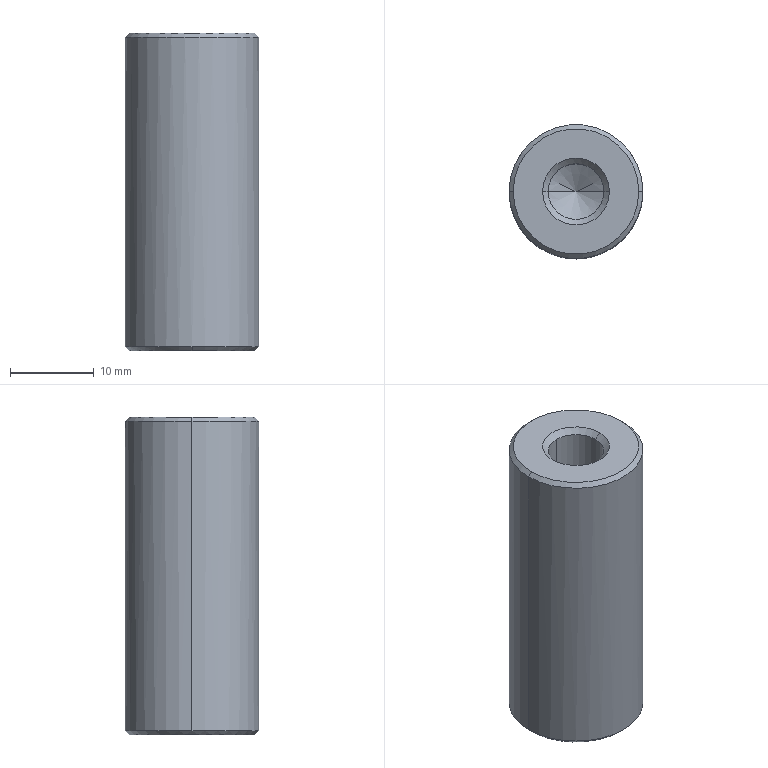Part | SolidWorks | features BaseBody 1 | 1 solid | 14 faces | box 16 x 16 x 38 mm | volume 7208 mm3 | cone 8 | cylinder 4 | plane 2 | commonest cylinder face diameters 6.647 x2 16 x2
STEP:
#1=CARTESIAN_POINT('',(0.,8.,-18.5));
#2=VERTEX_POINT('',#1);
#3=CARTESIAN_POINT('',(-8.,0.,-18.5));
#4=VERTEX_POINT('',#3);
#5=CARTESIAN_POINT('',(0.,0.,-18.5));
#6=DIRECTION('',(0.,0.,1.));
#7=DIRECTION('',(1.,0.,0.));
#8=AXIS2_PLACEMENT_3D('',#5,#6,#7);
#9=CIRCLE('',#8,8.);
#10=EDGE_CURVE('',#2,#4,#9,.T.);
#11=ORIENTED_EDGE('',*,*,#10,.T.);
#12=CARTESIAN_POINT('',(-8.,0.,18.5));
#13=VERTEX_POINT('',#12);
#14=CARTESIAN_POINT('',(-8.,0.,-19.));
#15=DIRECTION('',(0.,0.,1.));
#16=VECTOR('',#15,1000.);
#17=LINE('',#14,#16);
#18=EDGE_CURVE('',#4,#13,#17,.T.);
#19=ORIENTED_EDGE('',*,*,#18,.T.);
#20=CARTESIAN_POINT('',(8.,0.,18.5));
#21=VERTEX_POINT('',#20);
#22=CARTESIAN_POINT('',(0.,0.,18.5));
#23=DIRECTION('',(0.,0.,-1.));
#24=DIRECTION('',(1.,0.,0.));
#25=AXIS2_PLACEMENT_3D('',#22,#23,#24);
#26=CIRCLE('',#25,8.);
#27=EDGE_CURVE('',#13,#21,#26,.T.);
#28=ORIENTED_EDGE('',*,*,#27,.T.);
#29=CARTESIAN_POINT('',(8.,0.,-18.5));
#30=VERTEX_POINT('',#29);
#31=CARTESIAN_POINT('',(8.,0.,-19.));
#32=DIRECTION('',(0.,0.,1.));
#33=VECTOR('',#32,1000.);
#34=LINE('',#31,#33);
#35=EDGE_CURVE('',#30,#21,#34,.T.);
#36=ORIENTED_EDGE('',*,*,#35,.F.);
#37=CARTESIAN_POINT('',(0.,0.,-18.5));
#38=DIRECTION('',(0.,0.,1.));
#39=DIRECTION('',(1.,0.,0.));
#40=AXIS2_PLACEMENT_3D('',#37,#38,#39);
#41=CIRCLE('',#40,8.);
#42=EDGE_CURVE('',#30,#2,#41,.T.);
#43=ORIENTED_EDGE('',*,*,#42,.T.);
#44=EDGE_LOOP('',(#11,#19,#28,#36,#43));
#45=FACE_OUTER_BOUND('',#44,.T.);
#46=CARTESIAN_POINT('',(0.,0.,-19.));
#47=DIRECTION('',(0.,0.,1.));
#48=DIRECTION('',(1.,0.,0.));
#49=AXIS2_PLACEMENT_3D('',#46,#47,#48);
#50=CYLINDRICAL_SURFACE('',#49,8.);
#51=ADVANCED_FACE('',(#45),#50,.T.);
#52=CARTESIAN_POINT('',(-7.5,0.,19.));
#53=VERTEX_POINT('',#52);
#54=CARTESIAN_POINT('',(7.5,0.,19.));
#55=VERTEX_POINT('',#54);
#56=CARTESIAN_POINT('',(0.,0.,19.));
#57=DIRECTION('',(0.,0.,-1.));
#58=DIRECTION('',(-1.,0.,0.));
#59=AXIS2_PLACEMENT_3D('',#56,#57,#58);
#60=CIRCLE('',#59,7.5);
#61=EDGE_CURVE('',#53,#55,#60,.T.);
#62=ORIENTED_EDGE('',*,*,#61,.T.);
#63=CARTESIAN_POINT('',(8.,0.,18.5));
#64=DIRECTION('',(0.7071,0.,-0.7071));
#65=VECTOR('',#64,1000.);
#66=LINE('',#63,#65);
#67=EDGE_CURVE('',#55,#21,#66,.T.);
#68=ORIENTED_EDGE('',*,*,#67,.T.);
#69=ORIENTED_EDGE('',*,*,#27,.F.);
#70=CARTESIAN_POINT('',(-8.,0.,18.5));
#71=DIRECTION('',(-0.7071,0.,-0.7071));
#72=VECTOR('',#71,1000.);
#73=LINE('',#70,#72);
#74=EDGE_CURVE('',#53,#13,#73,.T.);
#75=ORIENTED_EDGE('',*,*,#74,.F.);
#76=EDGE_LOOP('',(#62,#68,#69,#75));
#77=FACE_OUTER_BOUND('',#76,.T.);
#78=CARTESIAN_POINT('',(0.,0.,18.5));
#79=DIRECTION('',(0.,0.,-1.));
#80=DIRECTION('',(-1.,0.,0.));
#81=AXIS2_PLACEMENT_3D('',#78,#79,#80);
#82=CONICAL_SURFACE('',#81,8.,0.7854);
#83=ADVANCED_FACE('',(#77),#82,.T.);
#84=CARTESIAN_POINT('',(0.,-7.5,-19.));
#85=VERTEX_POINT('',#84);
#86=CARTESIAN_POINT('',(0.,7.5,-19.));
#87=VERTEX_POINT('',#86);
#88=CARTESIAN_POINT('',(0.,0.,-19.));
#89=DIRECTION('',(0.,0.,1.));
#90=DIRECTION('',(0.,-1.,0.));
#91=AXIS2_PLACEMENT_3D('',#88,#89,#90);
#92=CIRCLE('',#91,7.5);
#93=EDGE_CURVE('',#85,#87,#92,.T.);
#94=ORIENTED_EDGE('',*,*,#93,.T.);
#95=CARTESIAN_POINT('',(0.,8.,-18.5));
#96=DIRECTION('',(0.,0.7071,0.7071));
#97=VECTOR('',#96,1000.);
#98=LINE('',#95,#97);
#99=EDGE_CURVE('',#87,#2,#98,.T.);
#100=ORIENTED_EDGE('',*,*,#99,.T.);
#101=ORIENTED_EDGE('',*,*,#42,.F.);
#102=CARTESIAN_POINT('',(0.,-8.,-18.5));
#103=VERTEX_POINT('',#102);
#104=CARTESIAN_POINT('',(0.,0.,-18.5));
#105=DIRECTION('',(0.,0.,1.));
#106=DIRECTION('',(1.,0.,0.));
#107=AXIS2_PLACEMENT_3D('',#104,#105,#106);
#108=CIRCLE('',#107,8.);
#109=EDGE_CURVE('',#103,#30,#108,.T.);
#110=ORIENTED_EDGE('',*,*,#109,.F.);
#111=CARTESIAN_POINT('',(0.,-8.,-18.5));
#112=DIRECTION('',(0.,-0.7071,0.7071));
#113=VECTOR('',#112,1000.);
#114=LINE('',#111,#113);
#115=EDGE_CURVE('',#85,#103,#114,.T.);
#116=ORIENTED_EDGE('',*,*,#115,.F.);
#117=EDGE_LOOP('',(#94,#100,#101,#110,#116));
#118=FACE_OUTER_BOUND('',#117,.T.);
#119=CARTESIAN_POINT('',(0.,0.,-18.5));
#120=DIRECTION('',(0.,0.,1.));
#121=DIRECTION('',(0.,-1.,0.));
#122=AXIS2_PLACEMENT_3D('',#119,#120,#121);
#123=CONICAL_SURFACE('',#122,8.,0.7854);
#124=ADVANCED_FACE('',(#118),#123,.T.);
#125=CARTESIAN_POINT('',(-3.323,0.,18.323));
#126=VERTEX_POINT('',#125);
#127=CARTESIAN_POINT('',(0.,-3.323,18.323));
#128=VERTEX_POINT('',#127);
#129=CARTESIAN_POINT('',(0.,0.,18.323));
#130=DIRECTION('',(0.,0.,1.));
#131=DIRECTION('',(0.,-1.,0.));
#132=AXIS2_PLACEMENT_3D('',#129,#130,#131);
#133=CIRCLE('',#132,3.323);
#134=EDGE_CURVE('',#126,#128,#133,.T.);
#135=ORIENTED_EDGE('',*,*,#134,.F.);
#136=CARTESIAN_POINT('',(-4.,0.,19.));
#137=VERTEX_POINT('',#136);
#138=CARTESIAN_POINT('',(-4.,0.,19.));
#139=DIRECTION('',(-0.7071,0.,0.7071));
#140=VECTOR('',#139,1000.);
#141=LINE('',#138,#140);
#142=EDGE_CURVE('',#126,#137,#141,.T.);
#143=ORIENTED_EDGE('',*,*,#142,.T.);
#144=CARTESIAN_POINT('',(4.,0.,19.));
#145=VERTEX_POINT('',#144);
#146=CARTESIAN_POINT('',(0.,0.,19.));
#147=DIRECTION('',(0.,0.,1.));
#148=DIRECTION('',(1.,0.,0.));
#149=AXIS2_PLACEMENT_3D('',#146,#147,#148);
#150=CIRCLE('',#149,4.);
#151=EDGE_CURVE('',#137,#145,#150,.T.);
#152=ORIENTED_EDGE('',*,*,#151,.T.);
#153=CARTESIAN_POINT('',(3.323,0.,18.323));
#154=VERTEX_POINT('',#153);
#155=CARTESIAN_POINT('',(4.,0.,19.));
#156=DIRECTION('',(0.7071,0.,0.7071));
#157=VECTOR('',#156,1000.);
#158=LINE('',#155,#157);
#159=EDGE_CURVE('',#154,#145,#158,.T.);
#160=ORIENTED_EDGE('',*,*,#159,.F.);
#161=CARTESIAN_POINT('',(0.,0.,18.323));
#162=DIRECTION('',(0.,0.,1.));
#163=DIRECTION('',(0.,-1.,0.));
#164=AXIS2_PLACEMENT_3D('',#161,#162,#163);
#165=CIRCLE('',#164,3.323);
#166=EDGE_CURVE('',#128,#154,#165,.T.);
#167=ORIENTED_EDGE('',*,*,#166,.F.);
#168=EDGE_LOOP('',(#135,#143,#152,#160,#167));
#169=FACE_OUTER_BOUND('',#168,.T.);
#170=CARTESIAN_POINT('',(0.,0.,19.));
#171=DIRECTION('',(0.,0.,1.));
#172=DIRECTION('',(1.,0.,0.));
#173=AXIS2_PLACEMENT_3D('',#170,#171,#172);
#174=CONICAL_SURFACE('',#173,4.,0.7854);
#175=ADVANCED_FACE('',(#169),#174,.F.);
#176=CARTESIAN_POINT('',(0.,3.323,7.676));
#177=VERTEX_POINT('',#176);
#178=CARTESIAN_POINT('',(-3.324,0.,7.676));
#179=VERTEX_POINT('',#178);
#180=CARTESIAN_POINT('',(0.,0.,7.676));
#181=DIRECTION('',(0.,0.,1.));
#182=DIRECTION('',(0.,-1.,0.));
#183=AXIS2_PLACEMENT_3D('',#180,#181,#182);
#184=CIRCLE('',#183,3.324);
#185=EDGE_CURVE('',#177,#179,#184,.T.);
#186=ORIENTED_EDGE('',*,*,#185,.F.);
#187=CARTESIAN_POINT('',(0.,3.323,18.323));
#188=VERTEX_POINT('',#187);
#189=CARTESIAN_POINT('',(0.,3.323,5.758));
#190=DIRECTION('',(0.,0.,1.));
#191=VECTOR('',#190,1000.);
#192=LINE('',#189,#191);
#193=EDGE_CURVE('',#177,#188,#192,.T.);
#194=ORIENTED_EDGE('',*,*,#193,.T.);
#195=CARTESIAN_POINT('',(0.,0.,18.323));
#196=DIRECTION('',(0.,0.,1.));
#197=DIRECTION('',(0.,-1.,0.));
#198=AXIS2_PLACEMENT_3D('',#195,#196,#197);
#199=CIRCLE('',#198,3.323);
#200=EDGE_CURVE('',#188,#126,#199,.T.);
#201=ORIENTED_EDGE('',*,*,#200,.T.);
#202=ORIENTED_EDGE('',*,*,#134,.T.);
#203=CARTESIAN_POINT('',(0.,-3.324,7.676));
#204=VERTEX_POINT('',#203);
#205=CARTESIAN_POINT('',(0.,-3.324,5.758));
#206=DIRECTION('',(0.,0.,1.));
#207=VECTOR('',#206,1000.);
#208=LINE('',#205,#207);
#209=EDGE_CURVE('',#204,#128,#208,.T.);
#210=ORIENTED_EDGE('',*,*,#209,.F.);
#211=CARTESIAN_POINT('',(0.,0.,7.676));
#212=DIRECTION('',(0.,0.,1.));
#213=DIRECTION('',(0.,-1.,0.));
#214=AXIS2_PLACEMENT_3D('',#211,#212,#213);
#215=CIRCLE('',#214,3.324);
#216=EDGE_CURVE('',#179,#204,#215,.T.);
#217=ORIENTED_EDGE('',*,*,#216,.F.);
#218=EDGE_LOOP('',(#186,#194,#201,#202,#210,#217));
#219=FACE_OUTER_BOUND('',#218,.T.);
#220=CARTESIAN_POINT('',(0.,0.,5.758));
#221=DIRECTION('',(0.,0.,1.));
#222=DIRECTION('',(0.,-1.,0.));
#223=AXIS2_PLACEMENT_3D('',#220,#221,#222);
#224=CYLINDRICAL_SURFACE('',#223,3.324);
#225=ADVANCED_FACE('',(#219),#224,.F.);
#226=CARTESIAN_POINT('',(0.,0.,5.758));
#227=VERTEX_POINT('',#226);
#228=CARTESIAN_POINT('',(3.324,0.,7.676));
#229=VERTEX_POINT('',#228);
#230=CARTESIAN_POINT('',(3.324,0.,7.677));
#231=DIRECTION('',(0.866,0.,0.5));
#232=VECTOR('',#231,1000.);
#233=LINE('',#230,#232);
#234=EDGE_CURVE('',#227,#229,#233,.T.);
#235=ORIENTED_EDGE('',*,*,#234,.F.);
#236=CARTESIAN_POINT('',(-3.324,0.,7.677));
#237=DIRECTION('',(-0.866,0.,0.5));
#238=VECTOR('',#237,1000.);
#239=LINE('',#236,#238);
#240=EDGE_CURVE('',#227,#179,#239,.T.);
#241=ORIENTED_EDGE('',*,*,#240,.T.);
#242=ORIENTED_EDGE('',*,*,#216,.T.);
#243=CARTESIAN_POINT('',(0.,0.,7.676));
#244=DIRECTION('',(0.,0.,1.));
#245=DIRECTION('',(0.,-1.,0.));
#246=AXIS2_PLACEMENT_3D('',#243,#244,#245);
#247=CIRCLE('',#246,3.324);
#248=EDGE_CURVE('',#204,#229,#247,.T.);
#249=ORIENTED_EDGE('',*,*,#248,.T.);
#250=EDGE_LOOP('',(#235,#241,#242,#249));
#251=FACE_OUTER_BOUND('',#250,.T.);
#252=CARTESIAN_POINT('',(0.,0.,7.677));
#253=DIRECTION('',(0.,0.,1.));
#254=DIRECTION('',(1.,0.,0.));
#255=AXIS2_PLACEMENT_3D('',#252,#253,#254);
#256=CONICAL_SURFACE('',#255,3.324,1.047);
#257=ADVANCED_FACE('',(#251),#256,.F.);
#258=ORIENTED_EDGE('',*,*,#18,.F.);
#259=CARTESIAN_POINT('',(0.,0.,-18.5));
#260=DIRECTION('',(0.,0.,1.));
#261=DIRECTION('',(1.,0.,0.));
#262=AXIS2_PLACEMENT_3D('',#259,#260,#261);
#263=CIRCLE('',#262,8.);
#264=EDGE_CURVE('',#4,#103,#263,.T.);
#265=ORIENTED_EDGE('',*,*,#264,.T.);
#266=ORIENTED_EDGE('',*,*,#109,.T.);
#267=ORIENTED_EDGE('',*,*,#35,.T.);
#268=CARTESIAN_POINT('',(0.,0.,18.5));
#269=DIRECTION('',(0.,0.,-1.));
#270=DIRECTION('',(1.,0.,0.));
#271=AXIS2_PLACEMENT_3D('',#268,#269,#270);
#272=CIRCLE('',#271,8.);
#273=EDGE_CURVE('',#21,#13,#272,.T.);
#274=ORIENTED_EDGE('',*,*,#273,.T.);
#275=EDGE_LOOP('',(#258,#265,#266,#267,#274));
#276=FACE_OUTER_BOUND('',#275,.T.);
#277=CARTESIAN_POINT('',(0.,0.,-19.));
#278=DIRECTION('',(0.,0.,1.));
#279=DIRECTION('',(1.,0.,0.));
#280=AXIS2_PLACEMENT_3D('',#277,#278,#279);
#281=CYLINDRICAL_SURFACE('',#280,8.);
#282=ADVANCED_FACE('',(#276),#281,.T.);
#283=ORIENTED_EDGE('',*,*,#67,.F.);
#284=CARTESIAN_POINT('',(0.,0.,19.));
#285=DIRECTION('',(0.,0.,-1.));
#286=DIRECTION('',(-1.,0.,0.));
#287=AXIS2_PLACEMENT_3D('',#284,#285,#286);
#288=CIRCLE('',#287,7.5);
#289=EDGE_CURVE('',#55,#53,#288,.T.);
#290=ORIENTED_EDGE('',*,*,#289,.T.);
#291=ORIENTED_EDGE('',*,*,#74,.T.);
#292=ORIENTED_EDGE('',*,*,#273,.F.);
#293=EDGE_LOOP('',(#283,#290,#291,#292));
#294=FACE_OUTER_BOUND('',#293,.T.);
#295=CARTESIAN_POINT('',(0.,0.,18.5));
#296=DIRECTION('',(0.,0.,-1.));
#297=DIRECTION('',(-1.,0.,0.));
#298=AXIS2_PLACEMENT_3D('',#295,#296,#297);
#299=CONICAL_SURFACE('',#298,8.,0.7854);
#300=ADVANCED_FACE('',(#294),#299,.T.);
#301=ORIENTED_EDGE('',*,*,#99,.F.);
#302=CARTESIAN_POINT('',(0.,0.,-19.));
#303=DIRECTION('',(0.,0.,1.));
#304=DIRECTION('',(0.,-1.,0.));
#305=AXIS2_PLACEMENT_3D('',#302,#303,#304);
#306=CIRCLE('',#305,7.5);
#307=EDGE_CURVE('',#87,#85,#306,.T.);
#308=ORIENTED_EDGE('',*,*,#307,.T.);
#309=ORIENTED_EDGE('',*,*,#115,.T.);
#310=ORIENTED_EDGE('',*,*,#264,.F.);
#311=ORIENTED_EDGE('',*,*,#10,.F.);
#312=EDGE_LOOP('',(#301,#308,#309,#310,#311));
#313=FACE_OUTER_BOUND('',#312,.T.);
#314=CARTESIAN_POINT('',(0.,0.,-18.5));
#315=DIRECTION('',(0.,0.,1.));
#316=DIRECTION('',(0.,-1.,0.));
#317=AXIS2_PLACEMENT_3D('',#314,#315,#316);
#318=CONICAL_SURFACE('',#317,8.,0.7854);
#319=ADVANCED_FACE('',(#313),#318,.T.);
#320=CARTESIAN_POINT('',(0.,0.,19.));
#321=DIRECTION('',(0.,0.,1.));
#322=DIRECTION('',(1.,0.,0.));
#323=AXIS2_PLACEMENT_3D('',#320,#321,#322);
#324=CIRCLE('',#323,4.);
#325=EDGE_CURVE('',#145,#137,#324,.T.);
#326=ORIENTED_EDGE('',*,*,#325,.F.);
#327=ORIENTED_EDGE('',*,*,#151,.F.);
#328=EDGE_LOOP('',(#326,#327));
#329=FACE_BOUND('',#328,.T.);
#330=ORIENTED_EDGE('',*,*,#61,.F.);
#331=ORIENTED_EDGE('',*,*,#289,.F.);
#332=EDGE_LOOP('',(#330,#331));
#333=FACE_OUTER_BOUND('',#332,.T.);
#334=CARTESIAN_POINT('',(0.,0.,19.));
#335=DIRECTION('',(0.,0.,-1.));
#336=DIRECTION('',(-1.,0.,0.));
#337=AXIS2_PLACEMENT_3D('',#334,#335,#336);
#338=PLANE('',#337);
#339=ADVANCED_FACE('',(#329,#333),#338,.F.);
#340=ORIENTED_EDGE('',*,*,#93,.F.);
#341=ORIENTED_EDGE('',*,*,#307,.F.);
#342=EDGE_LOOP('',(#340,#341));
#343=FACE_OUTER_BOUND('',#342,.T.);
#344=CARTESIAN_POINT('',(0.,7.5,-19.));
#345=DIRECTION('',(0.,0.,1.));
#346=DIRECTION('',(1.,0.,0.));
#347=AXIS2_PLACEMENT_3D('',#344,#345,#346);
#348=PLANE('',#347);
#349=ADVANCED_FACE('',(#343),#348,.F.);
#350=ORIENTED_EDGE('',*,*,#142,.F.);
#351=ORIENTED_EDGE('',*,*,#200,.F.);
#352=CARTESIAN_POINT('',(0.,0.,18.323));
#353=DIRECTION('',(0.,0.,1.));
#354=DIRECTION('',(0.,-1.,0.));
#355=AXIS2_PLACEMENT_3D('',#352,#353,#354);
#356=CIRCLE('',#355,3.323);
#357=EDGE_CURVE('',#154,#188,#356,.T.);
#358=ORIENTED_EDGE('',*,*,#357,.F.);
#359=ORIENTED_EDGE('',*,*,#159,.T.);
#360=ORIENTED_EDGE('',*,*,#325,.T.);
#361=EDGE_LOOP('',(#350,#351,#358,#359,#360));
#362=FACE_OUTER_BOUND('',#361,.T.);
#363=CARTESIAN_POINT('',(0.,0.,19.));
#364=DIRECTION('',(0.,0.,1.));
#365=DIRECTION('',(1.,0.,0.));
#366=AXIS2_PLACEMENT_3D('',#363,#364,#365);
#367=CONICAL_SURFACE('',#366,4.,0.7854);
#368=ADVANCED_FACE('',(#362),#367,.F.);
#369=ORIENTED_EDGE('',*,*,#193,.F.);
#370=CARTESIAN_POINT('',(0.,0.,7.676));
#371=DIRECTION('',(0.,0.,1.));
#372=DIRECTION('',(0.,-1.,0.));
#373=AXIS2_PLACEMENT_3D('',#370,#371,#372);
#374=CIRCLE('',#373,3.324);
#375=EDGE_CURVE('',#229,#177,#374,.T.);
#376=ORIENTED_EDGE('',*,*,#375,.F.);
#377=ORIENTED_EDGE('',*,*,#248,.F.);
#378=ORIENTED_EDGE('',*,*,#209,.T.);
#379=ORIENTED_EDGE('',*,*,#166,.T.);
#380=ORIENTED_EDGE('',*,*,#357,.T.);
#381=EDGE_LOOP('',(#369,#376,#377,#378,#379,#380));
#382=FACE_OUTER_BOUND('',#381,.T.);
#383=CARTESIAN_POINT('',(0.,0.,5.758));
#384=DIRECTION('',(0.,0.,1.));
#385=DIRECTION('',(0.,-1.,0.));
#386=AXIS2_PLACEMENT_3D('',#383,#384,#385);
#387=CYLINDRICAL_SURFACE('',#386,3.324);
#388=ADVANCED_FACE('',(#382),#387,.F.);
#389=ORIENTED_EDGE('',*,*,#240,.F.);
#390=ORIENTED_EDGE('',*,*,#234,.T.);
#391=ORIENTED_EDGE('',*,*,#375,.T.);
#392=ORIENTED_EDGE('',*,*,#185,.T.);
#393=EDGE_LOOP('',(#389,#390,#391,#392));
#394=FACE_OUTER_BOUND('',#393,.T.);
#395=CARTESIAN_POINT('',(0.,0.,7.677));
#396=DIRECTION('',(0.,0.,1.));
#397=DIRECTION('',(1.,0.,0.));
#398=AXIS2_PLACEMENT_3D('',#395,#396,#397);
#399=CONICAL_SURFACE('',#398,3.324,1.047);
#400=ADVANCED_FACE('',(#394),#399,.F.);
#401=CLOSED_SHELL('',(#51,#83,#124,#175,#225,#257,#282,#300,#319,#339,#349,#368,#388,#400));
#402=MANIFOLD_SOLID_BREP('',#401);
#403=CARTESIAN_POINT('',(0.,0.,0.));
#404=DIRECTION('',(0.,0.,1.));
#405=DIRECTION('',(1.,0.,0.));
#406=AXIS2_PLACEMENT_3D('',#403,#404,#405);
#407=(LENGTH_UNIT()NAMED_UNIT(*)SI_UNIT(.MILLI.,.METRE.));
#408=UNCERTAINTY_MEASURE_WITH_UNIT(LENGTH_MEASURE(0.00001),#407,'','');
#409=(NAMED_UNIT(*)PLANE_ANGLE_UNIT()SI_UNIT($,.RADIAN.));
#410=(NAMED_UNIT(*)SI_UNIT($,.STERADIAN.)SOLID_ANGLE_UNIT());
#411=(GEOMETRIC_REPRESENTATION_CONTEXT(3)GLOBAL_UNCERTAINTY_ASSIGNED_CONTEXT((#408))GLOBAL_UNIT_ASSIGNED_CONTEXT((#407,#409,#410))REPRESENTATION_CONTEXT('',''));
#412=ADVANCED_BREP_SHAPE_REPRESENTATION('',(#402,#406),#411);